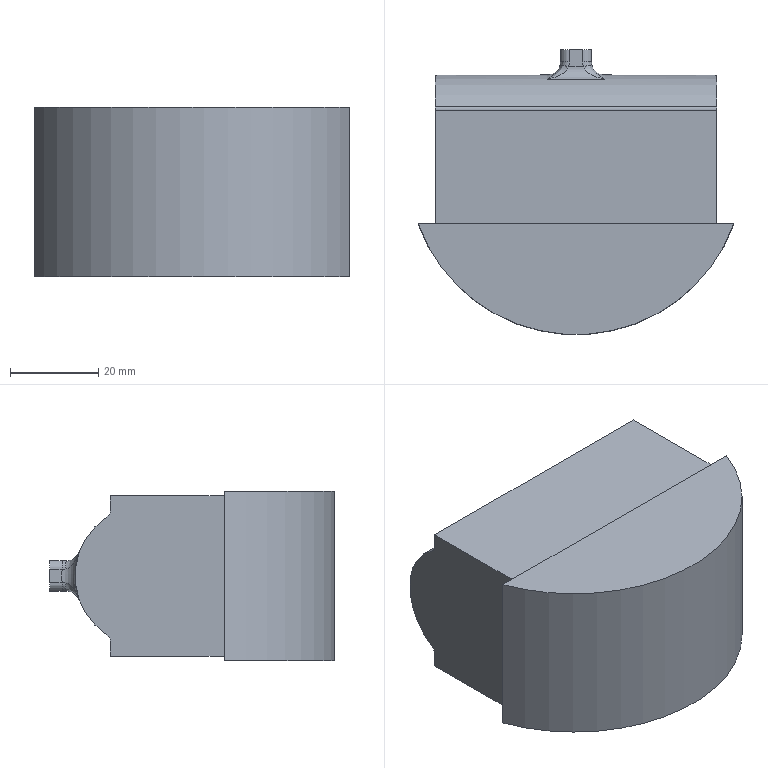NC program | NX | posted with a generic post | part box 71.627 x 64.667 x 38.42 mm
Lines 2471 to 3381 of 24266:
(ZLEVEL_PROFILE , TOOL : B4)
N4940 M6
N4942 G54
N4944 G17 G0 G90 X3.7 Y1.555 S3000 M3
N4946 G43 Z10. H0
N4948 Z0.2
N4950 G94 G1 Y-1.5 Z0.12 F2000.
N4952 Y-1.71 Z0.114
N4954 X3.594 Y-2.206 Z0.101
N4956 X3.377 Y-2.665 Z0.088
N4958 X3.062 Y-3.062 Z0.075
N4960 X2.665 Y-3.378 Z0.061
N4962 X2.206 Y-3.594 Z0.048
N4964 X1.71 Y-3.7 Z0.035
N4966 X0. Z-0.01
N4968 X-1.485 F2500.
N4970 X-1.5
N4972 G2 X-3.7 Y-1.5 R2.2
N4974 G1 Y1.5
N4976 G2 X-1.5 Y3.7 R2.2
N4978 G1 X1.485
N4980 X1.5
N4982 G2 X3.7 Y1.5 R2.2
N4984 G1 Y-1.5
N4986 G2 X1.5 Y-3.7 R2.2
N4988 G1 X0.
N4990 X-0.096 Y-3.723 Z-0.012
N4992 X-0.191 Y-3.744 Z-0.015
N4994 X-0.286 Y-3.764 Z-0.017
N4996 X-0.382 Y-3.782 Z-0.02
N4998 X-0.477 Y-3.799 Z-0.022
N5000 X-0.573 Y-3.815 Z-0.025
N5002 X-1.5
N5004 G2 X-3.815 Y-1.5 R2.315
N5006 G1 Y1.5
N5008 G2 X-1.5 Y3.815 R2.315
N5010 G1 X1.5
N5012 G2 X3.815 Y1.5 R2.315
N5014 G1 Y-1.5
N5016 G2 X1.5 Y-3.815 R2.315
N5018 G1 X0.
N5020 X-0.125 Y-3.835 Z-0.028
N5022 X-0.25 Y-3.854 Z-0.032
N5024 X-0.374 Y-3.871 Z-0.035
N5026 X-0.499 Y-3.888 Z-0.038
N5028 X-0.624 Y-3.904 Z-0.041
N5030 X-0.748 Y-3.92 Z-0.045
N5032 X-1.5
N5034 G2 X-3.92 Y-1.5 R2.42
N5036 G1 Y1.5
N5038 G2 X-1.5 Y3.92 R2.42
N5040 G1 X1.5
N5042 G2 X3.92 Y1.5 R2.42
N5044 G1 Y-1.5
N5046 G2 X1.5 Y-3.92 R2.42
N5048 G1 X0.
N5050 X-0.117 Y-3.934 Z-0.048
N5052 X-0.233 Y-3.947 Z-0.051
N5054 X-0.35 Y-3.96 Z-0.054
N5056 X-0.467 Y-3.973 Z-0.057
N5058 X-0.584 Y-3.986 Z-0.06
N5060 X-0.7 Y-3.998 Z-0.063
N5062 X-0.817 Y-4.009 Z-0.066
N5064 X-0.934 Y-4.021 Z-0.069
N5066 X-1.5
N5068 G2 X-4.021 Y-1.5 R2.521
N5070 G1 Y1.5
N5072 G2 X-1.5 Y4.021 R2.521
N5074 G1 X1.5
N5076 G2 X4.021 Y1.5 R2.521
N5078 G1 Y-1.5
N5080 G2 X1.5 Y-4.021 R2.521
N5082 G1 X0.
N5084 X-0.14 Y-4.034 Z-0.073
N5086 X-0.28 Y-4.047 Z-0.076
N5088 X-0.42 Y-4.06 Z-0.08
N5090 X-0.56 Y-4.072 Z-0.084
N5092 X-0.7 Y-4.085 Z-0.087
N5094 X-0.841 Y-4.096 Z-0.091
N5096 X-0.981 Y-4.108 Z-0.095
N5098 X-1.121 Y-4.119 Z-0.098
N5100 X-1.5
N5102 G2 X-4.119 Y-1.5 R2.619
N5104 G1 Y1.5
N5106 G2 X-1.5 Y4.119 R2.619
N5108 G1 X1.5
N5110 G2 X4.119 Y1.5 R2.619
N5112 G1 Y-1.5
N5114 G2 X1.5 Y-4.119 R2.619
N5116 G1 X0.
N5118 X-0.13 Y-4.13 Z-0.102
N5120 X-0.26 Y-4.14 Z-0.105
N5122 X-0.391 Y-4.15 Z-0.109
N5124 X-0.521 Y-4.16 Z-0.112
N5126 X-0.651 Y-4.17 Z-0.115
N5128 X-0.781 Y-4.179 Z-0.119
N5130 X-0.911 Y-4.188 Z-0.122
N5132 X-1.041 Y-4.198 Z-0.126
N5134 X-1.171 Y-4.207 Z-0.129
N5136 X-1.301 Y-4.216 Z-0.132
N5138 X-1.5
N5140 G2 X-4.216 Y-1.5 R2.716
N5142 G1 Y1.5
N5144 G2 X-1.5 Y4.216 R2.716
N5146 G1 X1.5
N5148 G2 X4.216 Y1.5 R2.716
N5150 G1 Y-1.5
N5152 G2 X1.5 Y-4.216 R2.716
N5154 G1 X0.
N5156 X-0.123 Y-4.224 Z-0.136
N5158 X-0.246 Y-4.232 Z-0.139
N5160 X-0.37 Y-4.24 Z-0.142
N5162 X-0.493 Y-4.248 Z-0.145
N5164 X-0.616 Y-4.256 Z-0.149
N5166 X-0.739 Y-4.264 Z-0.152
N5168 X-0.862 Y-4.272 Z-0.155
N5170 X-0.986 Y-4.28 Z-0.158
N5172 X-1.109 Y-4.287 Z-0.161
N5174 X-1.232 Y-4.295 Z-0.165
N5176 X-1.355 Y-4.302 Z-0.168
N5178 X-1.478 Y-4.309 Z-0.171
N5180 X-1.5
N5182 G2 X-4.309 Y-1.5 R2.809
N5184 G1 Y1.5
N5186 G2 X-1.5 Y4.309 R2.809
N5188 G1 X1.485
N5190 X1.5
N5192 G2 X4.309 Y1.5 R2.809
N5194 G1 Y-1.5
N5196 G2 X1.5 Y-4.309 R2.809
N5198 G1 X0.
N5200 X-0.138 Y-4.318 Z-0.175
N5202 X-0.276 Y-4.326 Z-0.178
N5204 X-0.413 Y-4.334 Z-0.182
N5206 X-0.551 Y-4.341 Z-0.186
N5208 X-0.689 Y-4.349 Z-0.189
N5210 X-0.827 Y-4.357 Z-0.193
N5212 X-0.965 Y-4.364 Z-0.196
N5214 X-1.102 Y-4.372 Z-0.2
N5216 X-1.24 Y-4.379 Z-0.204
N5218 X-1.378 Y-4.387 Z-0.207
N5220 X-1.518 Y-4.394 Z-0.211
N5222 X-1.658 Y-4.397 Z-0.214
N5224 G2 X-4.401 Y-1.5 R2.901
N5226 G1 Y1.5
N5228 G2 X-1.5 Y4.401 R2.901
N5230 G1 X1.5
N5232 G2 X4.401 Y1.5 R2.901
N5234 G1 Y-1.5
N5236 G2 X1.5 Y-4.401 R2.901
N5238 G1 X0.
N5240 X-0.13 Y-4.408 Z-0.218
N5242 X-0.26 Y-4.414 Z-0.221
N5244 X-0.391 Y-4.421 Z-0.225
N5246 X-0.521 Y-4.427 Z-0.228
N5248 X-0.651 Y-4.434 Z-0.231
N5250 X-0.781 Y-4.44 Z-0.235
N5252 X-0.911 Y-4.447 Z-0.238
N5254 X-1.041 Y-4.453 Z-0.242
N5256 X-1.172 Y-4.459 Z-0.245
N5258 X-1.302 Y-4.466 Z-0.249
N5260 X-1.433 Y-4.472 Z-0.252
N5262 X-1.564 Y-4.477 Z-0.255
N5264 X-1.698 Z-0.259
N5266 X-1.831 Y-4.471 Z-0.262
N5268 G2 X-4.49 Y-1.5 R2.99
N5270 G1 Y1.5
N5272 G2 X-1.5 Y4.49 R2.99
N5274 G1 X1.5
N5276 G2 X4.49 Y1.5 R2.99
N5278 G1 Y-1.5
N5280 G2 X1.5 Y-4.49 R2.99
N5282 G1 X0.
N5284 X-0.124 Y-4.496 Z-0.265
N5286 X-0.249 Y-4.501 Z-0.269
N5288 X-0.373 Y-4.507 Z-0.272
N5290 X-0.497 Y-4.512 Z-0.275
N5292 X-0.621 Y-4.518 Z-0.278
N5294 X-0.746 Y-4.523 Z-0.282
N5296 X-0.87 Y-4.529 Z-0.285
N5298 X-0.994 Y-4.534 Z-0.288
N5300 X-1.118 Y-4.54 Z-0.291
N5302 X-1.243 Y-4.545 Z-0.295
N5304 X-1.367 Y-4.55 Z-0.298
N5306 X-1.491 Y-4.555 Z-0.301
N5308 X-1.618 Y-4.558 Z-0.304
N5310 X-1.746 Y-4.556 Z-0.308
N5312 X-1.873 Y-4.548 Z-0.311
N5314 X-2. Y-4.535 Z-0.314
N5316 G2 X-4.576 Y-1.5 R3.076
N5318 G1 Y1.5
N5320 G2 X-1.5 Y4.576 R3.076
N5322 G1 X1.485
N5324 X1.5
N5326 G2 X4.576 Y1.5 R3.076
N5328 G1 Y-1.5
N5330 G2 X1.5 Y-4.576 R3.076
N5332 G1 X0.
N5334 X-0.134 Y-4.582 Z-0.318
N5336 X-0.269 Y-4.587 Z-0.321
N5338 X-0.403 Y-4.592 Z-0.325
N5340 X-0.537 Y-4.598 Z-0.328
N5342 X-0.671 Y-4.603 Z-0.332
N5344 X-0.806 Y-4.608 Z-0.335
N5346 X-0.94 Y-4.614 Z-0.339
N5348 X-1.074 Y-4.619 Z-0.342
N5350 X-1.208 Y-4.624 Z-0.346
N5352 X-1.343 Y-4.629 Z-0.349
N5354 X-1.478 Y-4.634 Z-0.353
N5356 X-1.613 Y-4.637 Z-0.356
N5358 X-1.751 Y-4.635 Z-0.36
N5360 X-1.888 Y-4.626 Z-0.363
N5362 X-2.025 Y-4.611 Z-0.367
N5364 X-2.161 Y-4.59 Z-0.37
N5366 G2 X-4.66 Y-1.5 R3.16
N5368 G1 Y1.5
N5370 G2 X-1.5 Y4.66 R3.16
N5372 G1 X1.5
N5374 G2 X4.66 Y1.5 R3.16
N5376 G1 Y-1.5
N5378 G2 X1.5 Y-4.66 R3.16
N5380 G1 X0.
N5382 X-0.128 Y-4.664 Z-0.374
N5384 X-0.256 Y-4.669 Z-0.377
N5386 X-0.384 Y-4.674 Z-0.38
N5388 X-0.512 Y-4.678 Z-0.384
N5390 X-0.64 Y-4.683 Z-0.387
N5392 X-0.768 Y-4.687 Z-0.391
N5394 X-0.896 Y-4.692 Z-0.394
N5396 X-1.024 Y-4.696 Z-0.397
N5398 X-1.152 Y-4.701 Z-0.401
N5400 X-1.28 Y-4.705 Z-0.404
N5402 X-1.408 Y-4.71 Z-0.407
N5404 X-1.536 Y-4.714 Z-0.411
N5406 X-1.667 Z-0.414
N5408 X-1.797 Y-4.709 Z-0.417
N5410 X-1.927 Y-4.699 Z-0.421
N5412 X-2.057 Y-4.683 Z-0.424
N5414 X-2.187 Y-4.662 Z-0.427
N5416 X-2.315 Y-4.636 Z-0.431
N5418 G2 X-4.74 Y-1.5 R3.24
N5420 G1 Y1.5
N5422 G2 X-1.5 Y4.74 R3.24
N5424 G1 X1.5
N5426 G2 X4.74 Y1.5 R3.24
N5428 G1 Y-1.5
N5430 G2 X1.5 Y-4.74 R3.24
N5432 G1 X0.
N5434 X-0.136 Y-4.744 Z-0.434
N5436 X-0.273 Y-4.749 Z-0.438
N5438 X-0.409 Y-4.753 Z-0.441
N5440 X-0.545 Y-4.758 Z-0.445
N5442 X-0.681 Y-4.762 Z-0.449
N5444 X-0.818 Y-4.767 Z-0.452
N5446 X-0.954 Y-4.771 Z-0.456
N5448 X-1.09 Y-4.775 Z-0.459
N5450 X-1.226 Y-4.78 Z-0.463
N5452 X-1.363 Y-4.784 Z-0.466
N5454 X-1.5 Y-4.788 Z-0.47
N5456 X-1.637 Y-4.789 Z-0.474
N5458 X-1.776 Y-4.785 Z-0.477
N5460 X-1.914 Y-4.775 Z-0.481
N5462 X-2.053 Y-4.758 Z-0.484
N5464 X-2.19 Y-4.736 Z-0.488
N5466 X-2.326 Y-4.708 Z-0.491
N5468 X-2.462 Y-4.675 Z-0.495
N5470 G2 X-4.817 Y-1.5 R3.317
N5472 G1 Y1.5
N5474 G2 X-1.5 Y4.817 R3.317
N5476 G1 X1.5
N5478 G2 X4.817 Y1.5 R3.317
N5480 G1 Y-1.5
N5482 G2 X1.5 Y-4.817 R3.317
N5484 G1 X0.
N5486 X-0.13 Y-4.821 Z-0.498
N5488 X-0.26 Y-4.825 Z-0.502
N5490 X-0.389 Y-4.829 Z-0.505
N5492 X-0.519 Y-4.833 Z-0.509
N5494 X-0.649 Y-4.836 Z-0.512
N5496 X-0.779 Y-4.84 Z-0.515
N5498 X-0.909 Y-4.844 Z-0.519
N5500 X-1.038 Y-4.848 Z-0.522
N5502 X-1.168 Y-4.851 Z-0.526
N5504 X-1.298 Y-4.855 Z-0.529
N5506 X-1.428 Y-4.859 Z-0.532
N5508 X-1.558 Y-4.862 Z-0.536
N5510 X-1.69 Y-4.861 Z-0.539
N5512 X-1.821 Y-4.854 Z-0.543
N5514 X-1.953 Y-4.843 Z-0.546
N5516 X-2.084 Y-4.826 Z-0.549
N5518 X-2.214 Y-4.804 Z-0.553
N5520 X-2.344 Y-4.777 Z-0.556
N5522 X-2.473 Y-4.745 Z-0.56
N5524 X-2.6 Y-4.708 Z-0.563
N5526 G2 X-4.891 Y-1.5 R3.391
N5528 G1 Y1.5
N5530 G2 X-1.5 Y4.891 R3.391
N5532 G1 X1.5
N5534 G2 X4.891 Y1.5 R3.391
N5536 G1 Y-1.5
N5538 G2 X1.5 Y-4.891 R3.391
N5540 G1 X0.
N5542 X-0.137 Y-4.895 Z-0.567
N5544 X-0.273 Y-4.898 Z-0.57
N5546 X-0.41 Y-4.902 Z-0.574
N5548 X-0.547 Y-4.906 Z-0.577
N5550 X-0.683 Y-4.909 Z-0.581
N5552 X-0.82 Y-4.913 Z-0.584
N5554 X-0.956 Y-4.916 Z-0.588
N5556 X-1.093 Y-4.92 Z-0.592
N5558 X-1.23 Y-4.924 Z-0.595
N5560 X-1.366 Y-4.927 Z-0.599
N5562 X-1.504 Y-4.931 Z-0.602
N5564 X-1.641 Z-0.606
N5566 X-1.78 Y-4.926 Z-0.609
N5568 X-1.918 Y-4.915 Z-0.613
N5570 X-2.056 Y-4.899 Z-0.617
N5572 X-2.193 Y-4.878 Z-0.62
N5574 X-2.329 Y-4.85 Z-0.624
N5576 X-2.464 Y-4.817 Z-0.627
N5578 X-2.598 Y-4.779 Z-0.631
N5580 X-2.73 Y-4.735 Z-0.634
N5582 G2 X-4.961 Y-1.5 R3.461
N5584 G1 Y1.5
N5586 G2 X-1.5 Y4.961 R3.461
N5588 G1 X1.5
N5590 G2 X4.961 Y1.5 R3.461
N5592 G1 Y-1.5
N5594 G2 X1.5 Y-4.961 R3.461
N5596 G1 X0.
N5598 X-0.13 Y-4.964 Z-0.638
N5600 X-0.26 Y-4.968 Z-0.641
N5602 X-0.39 Y-4.971 Z-0.645
N5604 X-0.52 Y-4.974 Z-0.648
N5606 X-0.651 Y-4.977 Z-0.652
N5608 X-0.781 Y-4.98 Z-0.655
N5610 X-0.911 Y-4.983 Z-0.658
N5612 X-1.041 Y-4.986 Z-0.662
N5614 X-1.171 Y-4.989 Z-0.665
N5616 X-1.301 Y-4.992 Z-0.669
N5618 X-1.431 Y-4.995 Z-0.672
N5620 X-1.562 Y-4.998 Z-0.675
N5622 X-1.693 Y-4.996 Z-0.679
N5624 X-1.825 Y-4.989 Z-0.682
N5626 X-1.956 Y-4.978 Z-0.686
N5628 X-2.087 Y-4.961 Z-0.689
N5630 X-2.217 Y-4.939 Z-0.692
N5632 X-2.347 Y-4.913 Z-0.696
N5634 X-2.475 Y-4.881 Z-0.699
N5636 X-2.602 Y-4.845 Z-0.703
N5638 X-2.728 Y-4.804 Z-0.706
N5640 X-2.853 Y-4.758 Z-0.709
N5642 G2 X-5.028 Y-1.5 R3.528
N5644 G1 Y1.5
N5646 G2 X-1.5 Y5.028 R3.528
N5648 G1 X1.5
N5650 G2 X5.028 Y1.5 R3.528
N5652 G1 Y-1.5
N5654 G2 X1.5 Y-5.028 R3.528
N5656 G1 X0.
N5658 X-0.136 Y-5.031 Z-0.713
N5660 X-0.271 Y-5.034 Z-0.717
N5662 X-0.407 Y-5.037 Z-0.72
N5664 X-0.543 Y-5.04 Z-0.724
N5666 X-0.679 Y-5.043 Z-0.727
N5668 X-0.814 Y-5.046 Z-0.731
N5670 X-0.95 Y-5.049 Z-0.734
N5672 X-1.086 Y-5.051 Z-0.738
N5674 X-1.221 Y-5.054 Z-0.741
N5676 X-1.357 Y-5.057 Z-0.745
N5678 X-1.493 Y-5.06 Z-0.749
N5680 X-1.63 Y-5.061 Z-0.752
N5682 X-1.767 Y-5.056 Z-0.756
N5684 X-1.903 Y-5.046 Z-0.759
N5686 X-2.04 Y-5.03 Z-0.763
N5688 X-2.176 Y-5.01 Z-0.766
N5690 X-2.311 Y-4.984 Z-0.77
N5692 X-2.445 Y-4.953 Z-0.773
N5694 X-2.578 Y-4.916 Z-0.777
N5696 X-2.709 Y-4.875 Z-0.78
N5698 X-2.839 Y-4.829 Z-0.784
N5700 X-2.967 Y-4.777 Z-0.788
N5702 G2 X-5.091 Y-1.5 R3.591
N5704 G1 Y1.5
N5706 G2 X-1.5 Y5.091 R3.591
N5708 G1 X1.5
N5710 G2 X5.091 Y1.5 R3.591
N5712 G1 Y-1.5
N5714 G2 X1.5 Y-5.091 R3.591
N5716 G1 X0.
N5718 X-0.141 Y-5.093 Z-0.791
N5720 X-0.282 Y-5.096 Z-0.795
N5722 X-0.423 Y-5.099 Z-0.799
N5724 X-0.564 Y-5.102 Z-0.802
N5726 X-0.705 Y-5.105 Z-0.806
N5728 X-0.846 Y-5.107 Z-0.81
N5730 X-0.986 Y-5.11 Z-0.813
N5732 X-1.127 Y-5.113 Z-0.817
N5734 X-1.268 Y-5.115 Z-0.821
N5736 X-1.409 Y-5.118 Z-0.824
N5738 X-1.551 Y-5.12 Z-0.828
N5740 X-1.693 Y-5.118 Z-0.832
N5742 X-1.835 Y-5.111 Z-0.836
N5744 X-1.977 Y-5.097 Z-0.839
N5746 X-2.118 Y-5.078 Z-0.843
N5748 X-2.258 Y-5.054 Z-0.847
N5750 X-2.398 Y-5.024 Z-0.85
N5752 X-2.536 Y-4.989 Z-0.854
N5754 X-2.673 Y-4.948 Z-0.858
N5756 X-2.808 Y-4.901 Z-0.861
N5758 X-2.942 Y-4.85 Z-0.865
N5760 X-3.073 Y-4.793 Z-0.869
N5762 G2 X-5.149 Y-1.5 R3.649
N5764 G1 Y1.5
N5766 G2 X-1.5 Y5.149 R3.649
N5768 G1 X1.5
N5770 G2 X5.149 Y1.5 R3.649
N5772 G1 Y-1.5
N5774 G2 X1.5 Y-5.149 R3.649
N5776 G1 X0.
N5778 X-0.134 Y-5.152 Z-0.872
N5780 X-0.267 Y-5.154 Z-0.876
N5782 X-0.401 Y-5.156 Z-0.879
N5784 X-0.535 Y-5.159 Z-0.883
N5786 X-0.668 Y-5.161 Z-0.886
N5788 X-0.802 Y-5.164 Z-0.89
N5790 X-0.936 Y-5.166 Z-0.893
N5792 X-1.069 Y-5.168 Z-0.897
N5794 X-1.203 Y-5.171 Z-0.9
N5796 X-1.337 Y-5.173 Z-0.904
N5798 X-1.471 Y-5.175 Z-0.907
N5800 X-1.605 Y-5.176 Z-0.911
N5802 X-1.74 Y-5.172 Z-0.914
N5804 X-1.874 Y-5.163 Z-0.918
N5806 X-2.008 Y-5.149 Z-0.921
N5808 X-2.142 Y-5.13 Z-0.925
N5810 X-2.275 Y-5.106 Z-0.928
N5812 X-2.407 Y-5.078 Z-0.932
N5814 X-2.538 Y-5.044 Z-0.935
N5816 X-2.668 Y-5.006 Z-0.939
N5818 X-2.796 Y-4.963 Z-0.942
N5820 X-2.923 Y-4.915 Z-0.946
N5822 X-3.048 Y-4.863 Z-0.949
N5824 X-3.171 Y-4.806 Z-0.953
N5826 G2 X-5.204 Y-1.5 R3.704
N5828 G1 Y1.5
N5830 G2 X-1.5 Y5.204 R3.704
N5832 G1 X1.5
N5834 G2 X5.204 Y1.5 R3.704
N5836 G1 Y-1.5
N5838 G2 X1.5 Y-5.204 R3.704
N5840 G1 X0.
N5842 X-0.138 Y-5.206 Z-0.956
N5844 X-0.276 Y-5.208 Z-0.96
N5846 X-0.414 Y-5.211 Z-0.964
N5848 X-0.551 Y-5.213 Z-0.967
N5850 X-0.689 Y-5.215 Z-0.971
N5852 X-0.827 Y-5.217 Z-0.974
N5854 X-0.965 Y-5.219 Z-0.978
N5856 X-1.102 Y-5.221 Z-0.982
N5858 X-1.24 Y-5.223 Z-0.985
N5860 X-1.378 Y-5.226 Z-0.989
N5862 X-1.516 Y-5.228 Z-0.992
N5864 X-1.655 Y-5.227 Z-0.996
N5866 X-1.793 Y-5.22 Z-1.
N5868 X-1.932 Y-5.209 Z-1.003
N5870 X-2.07 Y-5.192 Z-1.007
N5872 X-2.207 Y-5.171 Z-1.011
N5874 X-2.344 Y-5.144 Z-1.014
N5876 X-2.479 Y-5.112 Z-1.018
N5878 X-2.613 Y-5.075 Z-1.021
N5880 X-2.746 Y-5.033 Z-1.025
N5882 X-2.877 Y-4.986 Z-1.029
N5884 X-3.007 Y-4.934 Z-1.032
N5886 X-3.135 Y-4.877 Z-1.036
N5888 X-3.26 Y-4.816 Z-1.039
N5890 G2 X-5.254 Y-1.5 R3.754
N5892 G1 Y1.5
N5894 G2 X-1.5 Y5.254 R3.754
N5896 G1 X1.5
N5898 G2 X5.254 Y1.5 R3.754
N5900 G1 Y-1.5
N5902 G2 X1.5 Y-5.254 R3.754
N5904 G1 X0.
N5906 X-0.131 Y-5.256 Z-1.043
N5908 X-0.262 Y-5.258 Z-1.046
N5910 X-0.392 Y-5.26 Z-1.05
N5912 X-0.523 Y-5.262 Z-1.053
N5914 X-0.654 Y-5.263 Z-1.056
N5916 X-0.784 Y-5.265 Z-1.06
N5918 X-0.915 Y-5.267 Z-1.063
N5920 X-1.046 Y-5.269 Z-1.067
N5922 X-1.177 Y-5.271 Z-1.07
N5924 X-1.307 Y-5.273 Z-1.074
N5926 X-1.438 Y-5.274 Z-1.077
N5928 X-1.569 Y-5.275 Z-1.08
N5930 X-1.701 Y-5.273 Z-1.084
N5932 X-1.832 Y-5.265 Z-1.087
N5934 X-1.963 Y-5.253 Z-1.091
N5936 X-2.094 Y-5.236 Z-1.094
N5938 X-2.224 Y-5.215 Z-1.098
N5940 X-2.353 Y-5.189 Z-1.101
N5942 X-2.481 Y-5.159 Z-1.104
N5944 X-2.609 Y-5.124 Z-1.108
N5946 X-2.735 Y-5.085 Z-1.111
N5948 X-2.859 Y-5.041 Z-1.115
N5950 X-2.982 Y-4.994 Z-1.118
N5952 X-3.104 Y-4.941 Z-1.122
N5954 X-3.223 Y-4.885 Z-1.125
N5956 X-3.341 Y-4.824 Z-1.128
N5958 G2 X-5.3 Y-1.5 R3.8
N5960 G1 Y1.5
N5962 G2 X-1.5 Y5.3 R3.8
N5964 G1 X1.5
N5966 G2 X5.3 Y1.5 R3.8
N5968 G1 Y-1.5
N5970 G2 X1.5 Y-5.3 R3.8
N5972 G1 X0.
N5974 X-0.134 Y-5.302 Z-1.132
N5976 X-0.268 Y-5.303 Z-1.135
N5978 X-0.402 Y-5.305 Z-1.139
N5980 X-0.536 Y-5.307 Z-1.142
N5982 X-0.67 Y-5.308 Z-1.146
N5984 X-0.803 Y-5.31 Z-1.149
N5986 X-0.937 Y-5.312 Z-1.153
N5988 X-1.071 Y-5.313 Z-1.156
N5990 X-1.205 Y-5.315 Z-1.16
N5992 X-1.339 Y-5.317 Z-1.163
N5994 X-1.473 Y-5.318 Z-1.167
N5996 X-1.607 Z-1.17
N5998 X-1.742 Y-5.314 Z-1.174
N6000 X-1.876 Y-5.304 Z-1.177
N6002 X-2.01 Y-5.29 Z-1.181
N6004 X-2.144 Y-5.272 Z-1.184
N6006 X-2.277 Y-5.248 Z-1.188
N6008 X-2.408 Y-5.22 Z-1.191
N6010 X-2.539 Y-5.187 Z-1.195
N6012 X-2.669 Y-5.15 Z-1.198
N6014 X-2.798 Y-5.108 Z-1.202
N6016 X-2.924 Y-5.061 Z-1.206
N6018 X-3.05 Y-5.01 Z-1.209
N6020 X-3.173 Y-4.955 Z-1.213
N6022 X-3.294 Y-4.895 Z-1.216
N6024 X-3.413 Y-4.831 Z-1.22
N6026 G2 X-5.341 Y-1.5 R3.841
N6028 G1 Y1.5
N6030 G2 X-1.5 Y5.341 R3.841
N6032 G1 X1.5
N6034 G2 X5.341 Y1.5 R3.841
N6036 G1 Y-1.5
N6038 G2 X1.5 Y-5.341 R3.841
N6040 G1 X0.
N6042 X-0.137 Y-5.343 Z-1.223
N6044 X-0.274 Y-5.344 Z-1.227
N6046 X-0.41 Y-5.346 Z-1.23
N6048 X-0.547 Y-5.347 Z-1.234
N6050 X-0.684 Y-5.349 Z-1.237
N6052 X-0.821 Y-5.35 Z-1.241
N6054 X-0.957 Y-5.352 Z-1.245
N6056 X-1.094 Y-5.353 Z-1.248
N6058 X-1.231 Y-5.355 Z-1.252
N6060 X-1.368 Y-5.356 Z-1.255
N6062 X-1.505 Y-5.358 Z-1.259
N6064 X-1.642 Y-5.356 Z-1.262
N6066 X-1.779 Y-5.35 Z-1.266
N6068 X-1.916 Y-5.339 Z-1.27
N6070 X-2.053 Y-5.324 Z-1.273
N6072 X-2.189 Y-5.303 Z-1.277
N6074 X-2.324 Y-5.277 Z-1.28
N6076 X-2.458 Y-5.247 Z-1.284
N6078 X-2.591 Y-5.212 Z-1.288
N6080 X-2.723 Y-5.172 Z-1.291
N6082 X-2.853 Y-5.127 Z-1.295
N6084 X-2.982 Y-5.078 Z-1.298
N6086 X-3.109 Y-5.024 Z-1.302
N6088 X-3.234 Y-4.966 Z-1.305
N6090 X-3.357 Y-4.903 Z-1.309
N6092 X-3.478 Y-4.836 Z-1.313
N6094 G2 X-5.378 Y-1.5 R3.878
N6096 G1 Y1.5
N6098 G2 X-1.5 Y5.378 R3.878
N6100 G1 X1.5
N6102 G2 X5.378 Y1.5 R3.878
N6104 G1 Y-1.5
N6106 G2 X1.5 Y-5.378 R3.878
N6108 G1 X0.
N6110 X-0.139 Y-5.38 Z-1.316
N6112 X-0.279 Y-5.381 Z-1.32
N6114 X-0.418 Y-5.382 Z-1.324
N6116 X-0.557 Y-5.383 Z-1.327
N6118 X-0.696 Y-5.385 Z-1.331
N6120 X-0.836 Y-5.386 Z-1.335
N6122 X-0.975 Y-5.387 Z-1.338
N6124 X-1.114 Y-5.389 Z-1.342
N6126 X-1.253 Y-5.39 Z-1.345
N6128 X-1.393 Y-5.391 Z-1.349
N6130 X-1.532 Y-5.392 Z-1.353
N6132 X-1.672 Y-5.39 Z-1.356
N6134 X-1.811 Y-5.382 Z-1.36
N6136 X-1.951 Y-5.37 Z-1.364
N6138 X-2.09 Y-5.352 Z-1.367
N6140 X-2.228 Y-5.33 Z-1.371
N6142 X-2.365 Y-5.303 Z-1.375
N6144 X-2.501 Y-5.27 Z-1.378
N6146 X-2.636 Y-5.233 Z-1.382
N6148 X-2.77 Y-5.191 Z-1.386
N6150 X-2.902 Y-5.144 Z-1.389
N6152 X-3.032 Y-5.092 Z-1.393
N6154 X-3.161 Y-5.036 Z-1.396
N6156 X-3.287 Y-4.975 Z-1.4
N6158 X-3.411 Y-4.91 Z-1.404
N6160 X-3.533 Y-4.84 Z-1.407
N6162 G2 X-5.41 Y-1.5 R3.91
N6164 G1 Y1.5
N6166 G2 X-1.5 Y5.41 R3.91
N6168 G1 X1.5
N6170 G2 X5.41 Y1.5 R3.91
N6172 G1 Y-1.5
N6174 G2 X1.5 Y-5.41 R3.91
N6176 G1 X0.
N6178 X-0.131 Y-5.411 Z-1.411
N6180 X-0.263 Y-5.412 Z-1.414
N6182 X-0.394 Y-5.413 Z-1.418
N6184 X-0.525 Y-5.414 Z-1.421
N6186 X-0.657 Y-5.415 Z-1.425
N6188 X-0.788 Y-5.416 Z-1.428
N6190 X-0.919 Y-5.418 Z-1.432
N6192 X-1.051 Y-5.419 Z-1.435
N6194 X-1.182 Y-5.42 Z-1.438
N6196 X-1.313 Y-5.421 Z-1.442
N6198 X-1.445 Y-5.422 Z-1.445
N6200 X-1.576 Z-1.449
N6202 X-1.708 Y-5.418 Z-1.452
N6204 X-1.839 Y-5.41 Z-1.456
N6206 X-1.971 Y-5.397 Z-1.459
N6208 X-2.101 Y-5.38 Z-1.462
N6210 X-2.231 Y-5.359 Z-1.466
N6212 X-2.361 Y-5.333 Z-1.469
N6214 X-2.489 Y-5.303 Z-1.473
N6216 X-2.617 Y-5.268 Z-1.476
N6218 X-2.743 Y-5.23 Z-1.48
N6220 X-2.868 Y-5.187 Z-1.483
N6222 X-2.991 Y-5.139 Z-1.487
N6224 X-3.113 Y-5.088 Z-1.49
N6226 X-3.233 Y-5.033 Z-1.493
N6228 X-3.351 Y-4.973 Z-1.497
N6230 X-3.467 Y-4.91 Z-1.5
N6232 X-3.581 Y-4.843 Z-1.504
N6234 G2 X-5.437 Y-1.5 R3.937
N6236 G1 Y1.5
N6238 G2 X-1.5 Y5.437 R3.937
N6240 G1 X1.5
N6242 G2 X5.437 Y1.5 R3.937
N6244 G1 Y-1.5
N6246 G2 X1.5 Y-5.437 R3.937
N6248 G1 X0.
N6250 X-0.133 Y-5.438 Z-1.507
N6252 X-0.266 Y-5.439 Z-1.511
N6254 X-0.399 Y-5.44 Z-1.514
N6256 X-0.532 Y-5.441 Z-1.518
N6258 X-0.665 Y-5.442 Z-1.521
N6260 X-0.798 Y-5.443 Z-1.525
N6262 X-0.931 Y-5.444 Z-1.528
N6264 X-1.064 Z-1.532
N6266 X-1.197 Y-5.445 Z-1.535
N6268 X-1.33 Y-5.446 Z-1.539
N6270 X-1.463 Y-5.447 Z-1.542
N6272 X-1.596 Z-1.546
N6274 X-1.729 Y-5.442 Z-1.549
N6276 X-1.863 Y-5.433 Z-1.552
N6278 X-1.995 Y-5.419 Z-1.556
N6280 X-2.127 Y-5.401 Z-1.559
N6282 X-2.259 Y-5.378 Z-1.563
N6284 X-2.39 Y-5.351 Z-1.566
N6286 X-2.519 Y-5.32 Z-1.57
N6288 X-2.648 Y-5.284 Z-1.573
N6290 X-2.775 Y-5.243 Z-1.577
N6292 X-2.901 Y-5.199 Z-1.58
N6294 X-3.026 Y-5.15 Z-1.584
N6296 X-3.148 Y-5.097 Z-1.587
N6298 X-3.269 Y-5.04 Z-1.591
N6300 X-3.388 Y-4.979 Z-1.594
N6302 X-3.505 Y-4.914 Z-1.598
N6304 X-3.619 Y-4.845 Z-1.601
N6306 G2 X-5.46 Y-1.5 R3.96
N6308 G1 Y1.5
N6310 G2 X-1.5 Y5.46 R3.96
N6312 G1 X1.5
N6314 G2 X5.46 Y1.5 R3.96
N6316 G1 Y-1.5
N6318 G2 X1.5 Y-5.46 R3.96
N6320 G1 X0.
N6322 X-0.134 Y-5.461 Z-1.605
N6324 X-0.269 Z-1.608
N6326 X-0.403 Y-5.462 Z-1.612
N6328 X-0.537 Y-5.463 Z-1.615
N6330 X-0.672 Z-1.619
N6332 X-0.806 Y-5.464 Z-1.622
N6334 X-0.94 Y-5.465 Z-1.626
N6336 X-1.075 Z-1.629
N6338 X-1.209 Y-5.466 Z-1.633
N6340 X-1.343 Y-5.467 Z-1.636
N6342 X-1.478 Z-1.64
N6344 X-1.612 Y-5.466 Z-1.643
N6346 X-1.747 Y-5.461 Z-1.647
N6348 X-1.881 Y-5.451 Z-1.65
N6350 X-2.015 Y-5.436 Z-1.654
N6352 X-2.148 Y-5.417 Z-1.658
N6354 X-2.281 Y-5.394 Z-1.661
N6356 X-2.413 Y-5.365 Z-1.665
N6358 X-2.543 Y-5.333 Z-1.668
N6360 X-2.673 Y-5.296 Z-1.672
N6362 X-2.801 Y-5.254 Z-1.675
N6364 X-2.928 Y-5.209 Z-1.679
N6366 X-3.053 Y-5.159 Z-1.682
N6368 X-3.177 Y-5.104 Z-1.686
N6370 X-3.298 Y-5.046 Z-1.689
N6372 X-3.418 Y-4.983 Z-1.693
N6374 X-3.535 Y-4.917 Z-1.696
N6376 X-3.65 Y-4.846 Z-1.7
N6378 G2 X-5.477 Y-1.5 R3.977
N6380 G1 Y1.5
N6382 G2 X-1.5 Y5.477 R3.977
N6384 G1 X1.5
N6386 G2 X5.477 Y1.5 R3.977
N6388 G1 Y-1.5
N6390 G2 X1.5 Y-5.477 R3.977
N6392 G1 X0.
N6394 X-0.135 Y-5.478 Z-1.703
N6396 X-0.271 Z-1.707
N6398 X-0.406 Y-5.479 Z-1.71
N6400 X-0.541 Z-1.714
N6402 X-0.677 Y-5.48 Z-1.717
N6404 X-0.812 Z-1.721
N6406 X-0.947 Y-5.481 Z-1.725
N6408 X-1.083 Z-1.728
N6410 X-1.218 Y-5.482 Z-1.732
N6412 X-1.354 Z-1.735
N6414 X-1.489 Y-5.483 Z-1.739
N6416 X-1.624 Y-5.481 Z-1.742
N6418 X-1.76 Y-5.475 Z-1.746
N6420 X-1.895 Y-5.465 Z-1.749
N6422 X-2.03 Y-5.449 Z-1.753
N6424 X-2.164 Y-5.429 Z-1.756
N6426 X-2.297 Y-5.405 Z-1.76
N6428 X-2.43 Y-5.376 Z-1.764
N6430 X-2.561 Y-5.343 Z-1.767
N6432 X-2.691 Y-5.305 Z-1.771
N6434 X-2.82 Y-5.262 Z-1.774
N6436 X-2.948 Y-5.216 Z-1.778
N6438 X-3.073 Y-5.165 Z-1.781
N6440 X-3.197 Y-5.109 Z-1.785
N6442 X-3.319 Y-5.05 Z-1.788
N6444 X-3.439 Y-4.986 Z-1.792
N6446 X-3.557 Y-4.918 Z-1.795
N6448 X-3.672 Y-4.847 Z-1.799
N6450 G2 X-5.49 Y-1.5 R3.99
N6452 G1 Y1.5
N6454 G2 X-1.5 Y5.49 R3.99
N6456 G1 X1.5
N6458 G2 X5.49 Y1.5 R3.99
N6460 G1 Y-1.5
N6462 G2 X1.5 Y-5.49 R3.99
N6464 G1 X0.
N6466 X-0.136 Z-1.803
N6468 X-0.272 Y-5.491 Z-1.806
N6470 X-0.408 Z-1.81
N6472 X-0.544 Z-1.813
N6474 X-0.68 Y-5.492 Z-1.817
N6476 X-0.816 Z-1.82
N6478 X-0.952 Z-1.824
N6480 X-1.088 Y-5.493 Z-1.827
N6482 X-1.224 Z-1.831
N6484 X-1.36 Z-1.835
N6486 X-1.496 Z-1.838
N6488 X-1.632 Y-5.492 Z-1.842
N6490 X-1.768 Y-5.485 Z-1.845
N6492 X-1.904 Y-5.474 Z-1.849
N6494 X-2.039 Y-5.458 Z-1.852
N6496 X-2.174 Y-5.438 Z-1.856
N6498 X-2.308 Y-5.413 Z-1.859
N6500 X-2.44 Y-5.383 Z-1.863
N6502 X-2.572 Y-5.349 Z-1.867
N6504 X-2.703 Y-5.31 Z-1.87
N6506 X-2.832 Y-5.267 Z-1.874
N6508 X-2.96 Y-5.22 Z-1.877
N6510 X-3.086 Y-5.168 Z-1.881
N6512 X-3.21 Y-5.112 Z-1.884
N6514 X-3.332 Y-5.052 Z-1.888
N6516 X-3.452 Y-4.988 Z-1.892
N6518 X-3.57 Y-4.919 Z-1.895
N6520 X-3.686 Y-4.847 Z-1.899
N6522 G2 X-5.497 Y-1.5 R3.997
N6524 G1 Y1.5
N6526 G2 X-1.5 Y5.497 R3.997
N6528 G1 X1.5
N6530 G2 X5.497 Y1.5 R3.997
N6532 G1 Y-1.5
N6534 G2 X1.5 Y-5.497 R3.997
N6536 G1 X0.
N6538 X-0.136 Y-5.498 Z-1.902
N6540 X-0.272 Z-1.906
N6542 X-0.409 Z-1.909
N6544 X-0.545 Z-1.913
N6546 X-0.681 Z-1.916
N6548 X-0.817 Z-1.92
N6550 X-0.953 Y-5.499 Z-1.924
N6552 X-1.089 Z-1.927
N6554 X-1.225 Z-1.931
N6556 X-1.362 Z-1.934
N6558 X-1.498 Z-1.938
N6560 X-1.634 Y-5.497 Z-1.941
N6562 X-1.77 Y-5.49 Z-1.945
N6564 X-1.906 Y-5.479 Z-1.949
N6566 X-2.041 Y-5.463 Z-1.952
N6568 X-2.176 Y-5.442 Z-1.956
N6570 X-2.309 Y-5.417 Z-1.959
N6572 X-2.442 Y-5.387 Z-1.963
N6574 X-2.574 Y-5.353 Z-1.966
N6576 X-2.705 Y-5.314 Z-1.97
N6578 X-2.834 Y-5.271 Z-1.974
N6580 X-2.962 Y-5.223 Z-1.977
N6582 X-3.088 Y-5.171 Z-1.981
N6584 X-3.212 Y-5.115 Z-1.984
N6586 X-3.334 Y-5.055 Z-1.988
N6588 X-3.454 Y-4.99 Z-1.991
N6590 X-3.572 Y-4.922 Z-1.995
N6592 X-3.687 Y-4.849 Z-1.998
N6594 G2 X-5.467 Y-2.011 R4.
N6596 G1 X-5.472 Y-1.976
N6598 X-5.476 Y-1.941
N6600 X-5.5 Y-1.526
N6602 Y-1.5
N6604 Y1.5
N6606 Y1.54
N6608 X-5.486 Y1.795
N6610 X-5.485 Y1.843
N6612 X-5.472 Y1.976
N6614 X-5.467 Y1.993
N6616 X-5.455 Y2.082
N6618 Y2.1
N6620 G2 X-1.635 Y5.498 R4.
N6622 G1 X-1.568 Y5.499
N6624 X1.534 Y5.5
N6626 G2 X4.518 Y4.125 R4.008
N6628 X5.448 Y2.144 R3.993
N6630 G1 X5.467 Y2.011
N6632 X5.472 Y1.976
N6634 X5.481 Y1.888
N6636 X5.5 Y1.526
N6638 Y1.5
N6640 Y-1.5
N6642 Y-1.54
N6644 X5.474 Y-1.954
N6646 X5.472 Y-1.976
N6648 X5.468 Y-1.993
N6650 X5.455 Y-2.082
N6652 Y-2.1
N6654 G2 X1.624 Y-5.498 R4.
N6656 G1 X0.
N6658 X-0.137 Y-5.5 Z-2.002
N6660 X-1.364 Z-2.034
N6662 X-1.5 Z-2.038
N6664 X-1.637 Y-5.498 Z-2.041
N6666 X-1.773 Y-5.491 Z-2.045
N6668 X-1.909 Y-5.479 Z-2.048
N6670 X-2.044 Y-5.463 Z-2.052
N6672 X-2.179 Y-5.442 Z-2.056
N6674 X-2.313 Y-5.417 Z-2.059
N6676 X-2.446 Y-5.387 Z-2.063
N6678 X-2.578 Y-5.352 Z-2.066
N6680 X-2.709 Y-5.313 Z-2.07
N6682 X-2.838 Y-5.27 Z-2.073
N6684 X-2.966 Y-5.222 Z-2.077
N6686 X-3.092 Y-5.17 Z-2.081
N6688 X-3.216 Y-5.113 Z-2.084
N6690 X-3.338 Y-5.053 Z-2.088
N6692 X-3.458 Y-4.988 Z-2.091
N6694 X-3.576 Y-4.919 Z-2.095
N6696 X-3.691 Y-4.846 Z-2.098
N6698 G2 X-5.5 Y-1.5 R4.
N6700 G1 Y1.5
N6702 G2 X-1.5 Y5.5 R4.
N6704 G1 X1.5
N6706 G2 X5.5 Y1.5 R4.
N6708 G1 Y-1.5
N6710 G2 X1.5 Y-5.5 R4.
N6712 G1 X0.
N6714 X-1.364 Z-2.134
N6716 X-1.5 Z-2.138
N6718 X-1.637 Y-5.498 Z-2.141
N6720 X-1.773 Y-5.491 Z-2.145
N6722 X-1.909 Y-5.479 Z-2.148
N6724 X-2.044 Y-5.463 Z-2.152
N6726 X-2.179 Y-5.442 Z-2.156
N6728 X-2.313 Y-5.417 Z-2.159
N6730 X-2.446 Y-5.387 Z-2.163
N6732 X-2.578 Y-5.352 Z-2.166
N6734 X-2.709 Y-5.313 Z-2.17
N6736 X-2.838 Y-5.27 Z-2.173
N6738 X-2.966 Y-5.222 Z-2.177
N6740 X-3.092 Y-5.17 Z-2.181
N6742 X-3.216 Y-5.113 Z-2.184
N6744 X-3.338 Y-5.053 Z-2.188
N6746 X-3.458 Y-4.988 Z-2.191
N6748 X-3.576 Y-4.919 Z-2.195
N6750 X-3.691 Y-4.846 Z-2.198
N6752 G2 X-5.5 Y-1.5 R4.
N6754 G1 Y1.5